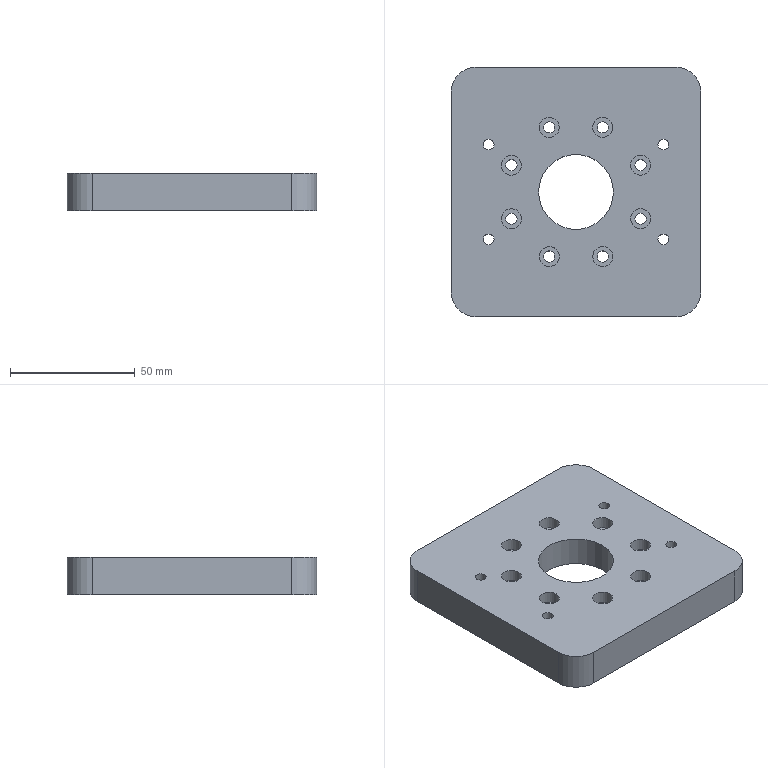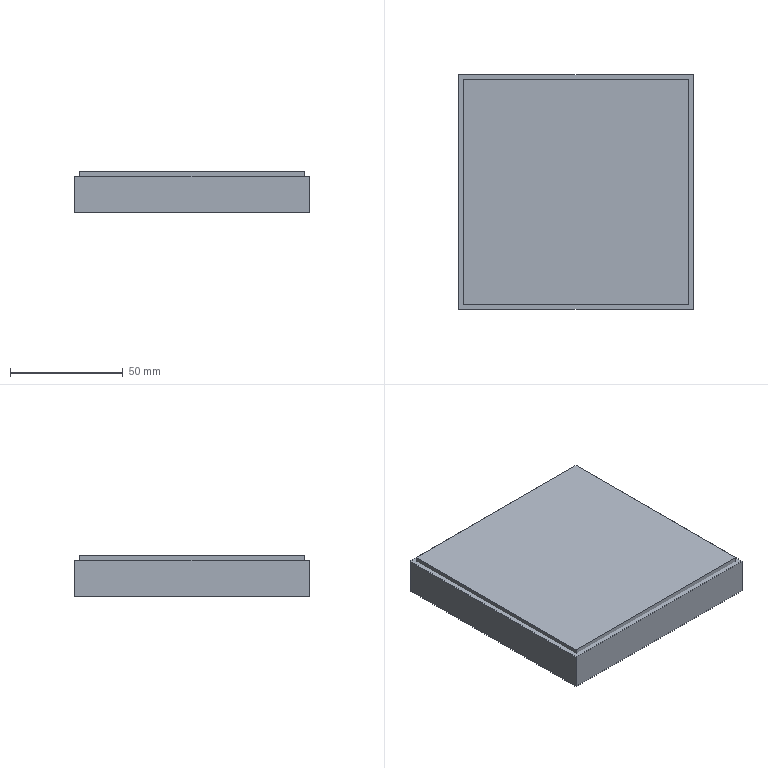CAM job | NX | 3-axis milling, drilling | part box 100 x 100 x 15 mm | stock box 104 x 104 x 18 mm
Tools:
number,name,description,diameter,corner_radius,flute_length,length,flutes
1,D63,Milling Tool-5 Parameters,63.0,0.0,50.0,75.0,2
10,D10,Milling Tool-5 Parameters,10.0,0.0,50.0,75.0,2
7,D6A45,Milling Tool-5 Parameters,6.0,0.0,50.0,75.0,2
14,4.3ZT,Drilling Tool,4.3,0.0,35.0,50.0,2
15,4.5ZT,Drilling Tool,4.5,0.0,35.0,50.0,2
6,D6,Milling Tool-5 Parameters,6.0,0.0,50.0,75.0,2
Operations:
program,operation,operation_type,tool,method,geometry_group,spindle_rpm,surface_speed,feed_per_tooth,feed_cut,feed_plunge,cut_length_mm,path_length_mm,cut_time_min,machine_time_min
1,FLOOR_WALL_1,VolumeBased25DMillingOperation,D63,METHOD,A,6500.0,1286.0,0.1154,1500.0,100.0,758.797,812.797,0.5059,0.5113
1,ZLEVEL_PROFILE,ZLevelMilling,D10,METHOD,A,9500.0,298.0,0.1842,3500.0,1000.0,6687.101,6759.101,1.945,1.952
1,ZLEVEL_PROFILE_COPY,ZLevelMilling,D10,METHOD,A,9500.0,298.0,0.0789,1500.0,1000.0,422.71,509.71,0.2832,0.2919
1,HOLE_MILLING,CylinderMilling,D10,METHOD,A,9500.0,0.0,0.0,2200.0,100.0,1586.564,1676.564,0.7212,0.7302
1,HOLE_MILLING_COPY,CylinderMilling,D10,METHOD,A,9500.0,0.0,0.0632,1200.0,100.0,185.377,259.877,0.1545,0.1619
1,DRILLING,Operation,D6A45,METHOD,A,5000.0,94.0,0.025,250.0,0.0,52.0,441.72,0.208,0.247
1,DRILLING_COPY,Operation,4.3ZT,METHOD,A,2000.0,31.0,0.0625,250.0,0.0,83.167,381.635,0.3327,0.3625
1,DRILLING_COPY_COPY,Operation,4.5ZT,METHOD,A,2000.0,31.0,0.0625,250.0,0.0,154.815,542.106,0.6193,0.658
1,HOLE_MILLING_1,CylinderMilling,D6,METHOD,A,9500.0,179.0,0.0789,1500.0,100.0,630.067,1296.078,0.42,0.4866
1,PLANAR_MILL,PlanarMilling,D6A45,METHOD,A,9500.0,179.0,0.0658,1250.0,100.0,735.64,1851.177,0.5885,0.7001
2,FLOOR_WALL_1_COPY,VolumeBased25DMillingOperation,D63,METHOD,B,6500.0,1286.0,0.1154,1500.0,100.0,2216.391,2521.986,1.478,1.508
2,HOLE_MILLING_COPY_1,CylinderMilling,D10,METHOD,B,9500.0,0.0,0.0,2200.0,100.0,2756.407,2832.907,1.253,1.261
2,10,CylinderMilling,D10,METHOD,B,9500.0,0.0,0.0632,1200.0,100.0,364.562,427.062,0.3038,0.3101
2,PLANAR_MILL_COPY,PlanarMilling,D6A45,METHOD,B,9500.0,179.0,0.0658,1250.0,100.0,639.907,1202.112,0.5119,0.5681
2,PLANAR_MILL_COPY_COPY,PlanarMilling,D6A45,METHOD,B,9500.0,179.0,0.0658,1250.0,100.0,93.687,158.687,0.0749,0.0814